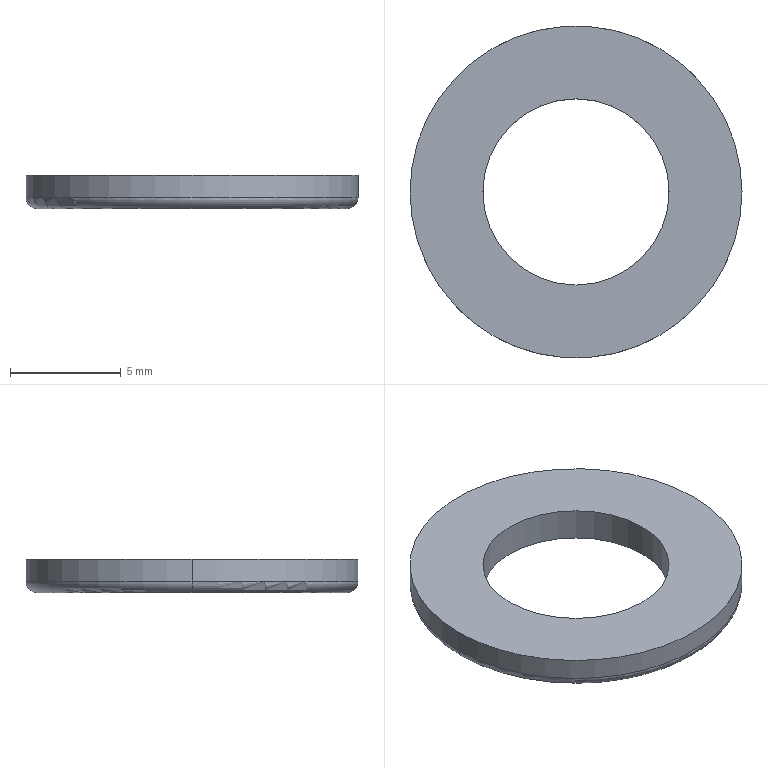Part | NX | features BREP 1 | 1 solid | 8 faces | box 15 x 15 x 1.5 mm | volume 179.214 mm3 | cylinder 4 | torus 2 | plane 2 | commonest cylinder face diameters 8.412 x2 15 x2
STEP:
#1=CARTESIAN_POINT('',(7.5,0.,6.));
#2=VERTEX_POINT('',#1);
#3=CARTESIAN_POINT('',(-7.5,0.,6.));
#4=VERTEX_POINT('',#3);
#5=CARTESIAN_POINT('',(0.,0.,6.));
#6=DIRECTION('',(0.,0.,-1.));
#7=DIRECTION('',(1.,0.,0.));
#8=AXIS2_PLACEMENT_3D('',#5,#6,#7);
#9=CIRCLE('',#8,7.5);
#10=EDGE_CURVE('',#2,#4,#9,.T.);
#11=ORIENTED_EDGE('',*,*,#10,.F.);
#12=CARTESIAN_POINT('',(7.5,0.,7.));
#13=VERTEX_POINT('',#12);
#14=CARTESIAN_POINT('',(7.5,0.,7.));
#15=DIRECTION('',(0.,0.,-1.));
#16=VECTOR('',#15,1000.);
#17=LINE('',#14,#16);
#18=EDGE_CURVE('',#13,#2,#17,.T.);
#19=ORIENTED_EDGE('',*,*,#18,.F.);
#20=CARTESIAN_POINT('',(-7.5,0.,7.));
#21=VERTEX_POINT('',#20);
#22=CARTESIAN_POINT('',(0.,0.,7.));
#23=DIRECTION('',(0.,0.,1.));
#24=DIRECTION('',(-1.,0.,0.));
#25=AXIS2_PLACEMENT_3D('',#22,#23,#24);
#26=CIRCLE('',#25,7.5);
#27=EDGE_CURVE('',#21,#13,#26,.T.);
#28=ORIENTED_EDGE('',*,*,#27,.F.);
#29=CARTESIAN_POINT('',(-7.5,0.,7.));
#30=DIRECTION('',(0.,0.,-1.));
#31=VECTOR('',#30,1000.);
#32=LINE('',#29,#31);
#33=EDGE_CURVE('',#21,#4,#32,.T.);
#34=ORIENTED_EDGE('',*,*,#33,.T.);
#35=EDGE_LOOP('',(#11,#19,#28,#34));
#36=FACE_BOUND('',#35,.T.);
#37=CARTESIAN_POINT('',(0.,0.,5.5));
#38=DIRECTION('',(0.,0.,1.));
#39=DIRECTION('',(-1.,0.,0.));
#40=AXIS2_PLACEMENT_3D('',#37,#38,#39);
#41=CYLINDRICAL_SURFACE('',#40,7.5);
#42=ADVANCED_FACE('',(#36),#41,.T.);
#43=ORIENTED_EDGE('',*,*,#33,.F.);
#44=CARTESIAN_POINT('',(0.,0.,7.));
#45=DIRECTION('',(0.,0.,1.));
#46=DIRECTION('',(1.,0.,0.));
#47=AXIS2_PLACEMENT_3D('',#44,#45,#46);
#48=CIRCLE('',#47,7.5);
#49=EDGE_CURVE('',#13,#21,#48,.T.);
#50=ORIENTED_EDGE('',*,*,#49,.F.);
#51=ORIENTED_EDGE('',*,*,#18,.T.);
#52=CARTESIAN_POINT('',(0.,0.,6.));
#53=DIRECTION('',(0.,0.,-1.));
#54=DIRECTION('',(-1.,0.,0.));
#55=AXIS2_PLACEMENT_3D('',#52,#53,#54);
#56=CIRCLE('',#55,7.5);
#57=EDGE_CURVE('',#4,#2,#56,.T.);
#58=ORIENTED_EDGE('',*,*,#57,.F.);
#59=EDGE_LOOP('',(#43,#50,#51,#58));
#60=FACE_BOUND('',#59,.T.);
#61=CARTESIAN_POINT('',(0.,0.,5.5));
#62=DIRECTION('',(0.,0.,1.));
#63=DIRECTION('',(-1.,0.,0.));
#64=AXIS2_PLACEMENT_3D('',#61,#62,#63);
#65=CYLINDRICAL_SURFACE('',#64,7.5);
#66=ADVANCED_FACE('',(#60),#65,.T.);
#67=CARTESIAN_POINT('',(7.,0.,5.5));
#68=VERTEX_POINT('',#67);
#69=CARTESIAN_POINT('',(7.,0.,6.));
#70=DIRECTION('',(0.,-1.,0.));
#71=DIRECTION('',(0.,0.,-1.));
#72=AXIS2_PLACEMENT_3D('',#69,#70,#71);
#73=CIRCLE('',#72,0.5);
#74=EDGE_CURVE('',#68,#2,#73,.T.);
#75=ORIENTED_EDGE('',*,*,#74,.F.);
#76=CARTESIAN_POINT('',(-7.,0.,5.5));
#77=VERTEX_POINT('',#76);
#78=CARTESIAN_POINT('',(0.,0.,5.5));
#79=DIRECTION('',(0.,0.,-1.));
#80=DIRECTION('',(-1.,0.,0.));
#81=AXIS2_PLACEMENT_3D('',#78,#79,#80);
#82=CIRCLE('',#81,7.);
#83=EDGE_CURVE('',#77,#68,#82,.T.);
#84=ORIENTED_EDGE('',*,*,#83,.F.);
#85=CARTESIAN_POINT('',(-7.,0.,6.));
#86=DIRECTION('',(0.,1.,0.));
#87=DIRECTION('',(0.,0.,-1.));
#88=AXIS2_PLACEMENT_3D('',#85,#86,#87);
#89=CIRCLE('',#88,0.5);
#90=EDGE_CURVE('',#77,#4,#89,.T.);
#91=ORIENTED_EDGE('',*,*,#90,.T.);
#92=ORIENTED_EDGE('',*,*,#57,.T.);
#93=EDGE_LOOP('',(#75,#84,#91,#92));
#94=FACE_BOUND('',#93,.T.);
#95=CARTESIAN_POINT('',(0.,0.,6.));
#96=DIRECTION('',(0.,0.,-1.));
#97=DIRECTION('',(1.,0.,0.));
#98=AXIS2_PLACEMENT_3D('',#95,#96,#97);
#99=TOROIDAL_SURFACE('',#98,7.,0.5);
#100=ADVANCED_FACE('',(#94),#99,.T.);
#101=ORIENTED_EDGE('',*,*,#10,.T.);
#102=ORIENTED_EDGE('',*,*,#90,.F.);
#103=CARTESIAN_POINT('',(0.,0.,5.5));
#104=DIRECTION('',(0.,0.,-1.));
#105=DIRECTION('',(1.,0.,0.));
#106=AXIS2_PLACEMENT_3D('',#103,#104,#105);
#107=CIRCLE('',#106,7.);
#108=EDGE_CURVE('',#68,#77,#107,.T.);
#109=ORIENTED_EDGE('',*,*,#108,.F.);
#110=ORIENTED_EDGE('',*,*,#74,.T.);
#111=EDGE_LOOP('',(#101,#102,#109,#110));
#112=FACE_BOUND('',#111,.T.);
#113=CARTESIAN_POINT('',(0.,0.,6.));
#114=DIRECTION('',(0.,0.,-1.));
#115=DIRECTION('',(1.,0.,0.));
#116=AXIS2_PLACEMENT_3D('',#113,#114,#115);
#117=TOROIDAL_SURFACE('',#116,7.,0.5);
#118=ADVANCED_FACE('',(#112),#117,.T.);
#119=ORIENTED_EDGE('',*,*,#108,.T.);
#120=ORIENTED_EDGE('',*,*,#83,.T.);
#121=EDGE_LOOP('',(#119,#120));
#122=FACE_BOUND('',#121,.T.);
#123=CARTESIAN_POINT('',(4.206,0.,5.5));
#124=VERTEX_POINT('',#123);
#125=CARTESIAN_POINT('',(-4.206,0.,5.5));
#126=VERTEX_POINT('',#125);
#127=CARTESIAN_POINT('',(0.,0.,5.5));
#128=DIRECTION('',(0.,0.,1.));
#129=DIRECTION('',(1.,0.,0.));
#130=AXIS2_PLACEMENT_3D('',#127,#128,#129);
#131=CIRCLE('',#130,4.206);
#132=EDGE_CURVE('',#124,#126,#131,.T.);
#133=ORIENTED_EDGE('',*,*,#132,.T.);
#134=CARTESIAN_POINT('',(0.,0.,5.5));
#135=DIRECTION('',(0.,0.,1.));
#136=DIRECTION('',(-1.,0.,0.));
#137=AXIS2_PLACEMENT_3D('',#134,#135,#136);
#138=CIRCLE('',#137,4.206);
#139=EDGE_CURVE('',#126,#124,#138,.T.);
#140=ORIENTED_EDGE('',*,*,#139,.T.);
#141=EDGE_LOOP('',(#133,#140));
#142=FACE_BOUND('',#141,.T.);
#143=CARTESIAN_POINT('',(0.,0.,5.5));
#144=DIRECTION('',(0.,0.,-1.));
#145=DIRECTION('',(1.,0.,0.));
#146=AXIS2_PLACEMENT_3D('',#143,#144,#145);
#147=PLANE('',#146);
#148=ADVANCED_FACE('',(#122,#142),#147,.T.);
#149=CARTESIAN_POINT('',(-4.206,0.,7.));
#150=VERTEX_POINT('',#149);
#151=CARTESIAN_POINT('',(-4.206,0.,7.));
#152=DIRECTION('',(0.,0.,-1.));
#153=VECTOR('',#152,1000.);
#154=LINE('',#151,#153);
#155=EDGE_CURVE('',#126,#150,#154,.F.);
#156=ORIENTED_EDGE('',*,*,#155,.T.);
#157=CARTESIAN_POINT('',(4.206,0.,7.));
#158=VERTEX_POINT('',#157);
#159=CARTESIAN_POINT('',(0.,0.,7.));
#160=DIRECTION('',(0.,0.,-1.));
#161=DIRECTION('',(1.,0.,0.));
#162=AXIS2_PLACEMENT_3D('',#159,#160,#161);
#163=CIRCLE('',#162,4.206);
#164=EDGE_CURVE('',#158,#150,#163,.T.);
#165=ORIENTED_EDGE('',*,*,#164,.F.);
#166=CARTESIAN_POINT('',(4.206,0.,7.));
#167=DIRECTION('',(0.,0.,-1.));
#168=VECTOR('',#167,1000.);
#169=LINE('',#166,#168);
#170=EDGE_CURVE('',#124,#158,#169,.F.);
#171=ORIENTED_EDGE('',*,*,#170,.F.);
#172=ORIENTED_EDGE('',*,*,#139,.F.);
#173=EDGE_LOOP('',(#156,#165,#171,#172));
#174=FACE_BOUND('',#173,.T.);
#175=CARTESIAN_POINT('',(0.,0.,5.5));
#176=DIRECTION('',(0.,0.,1.));
#177=DIRECTION('',(-1.,0.,0.));
#178=AXIS2_PLACEMENT_3D('',#175,#176,#177);
#179=CYLINDRICAL_SURFACE('',#178,4.206);
#180=ADVANCED_FACE('',(#174),#179,.F.);
#181=ORIENTED_EDGE('',*,*,#132,.F.);
#182=ORIENTED_EDGE('',*,*,#170,.T.);
#183=CARTESIAN_POINT('',(0.,0.,7.));
#184=DIRECTION('',(0.,0.,-1.));
#185=DIRECTION('',(-1.,0.,0.));
#186=AXIS2_PLACEMENT_3D('',#183,#184,#185);
#187=CIRCLE('',#186,4.206);
#188=EDGE_CURVE('',#150,#158,#187,.T.);
#189=ORIENTED_EDGE('',*,*,#188,.F.);
#190=ORIENTED_EDGE('',*,*,#155,.F.);
#191=EDGE_LOOP('',(#181,#182,#189,#190));
#192=FACE_BOUND('',#191,.T.);
#193=CARTESIAN_POINT('',(0.,0.,5.5));
#194=DIRECTION('',(0.,0.,1.));
#195=DIRECTION('',(-1.,0.,0.));
#196=AXIS2_PLACEMENT_3D('',#193,#194,#195);
#197=CYLINDRICAL_SURFACE('',#196,4.206);
#198=ADVANCED_FACE('',(#192),#197,.F.);
#199=ORIENTED_EDGE('',*,*,#49,.T.);
#200=ORIENTED_EDGE('',*,*,#27,.T.);
#201=EDGE_LOOP('',(#199,#200));
#202=FACE_BOUND('',#201,.T.);
#203=ORIENTED_EDGE('',*,*,#188,.T.);
#204=ORIENTED_EDGE('',*,*,#164,.T.);
#205=EDGE_LOOP('',(#203,#204));
#206=FACE_BOUND('',#205,.T.);
#207=CARTESIAN_POINT('',(0.,0.,7.));
#208=DIRECTION('',(0.,0.,-1.));
#209=DIRECTION('',(1.,0.,0.));
#210=AXIS2_PLACEMENT_3D('',#207,#208,#209);
#211=PLANE('',#210);
#212=ADVANCED_FACE('',(#202,#206),#211,.F.);
#213=CLOSED_SHELL('',(#42,#66,#100,#118,#148,#180,#198,#212));
#214=MANIFOLD_SOLID_BREP('',#213);
#215=(LENGTH_UNIT()NAMED_UNIT(*)SI_UNIT(.MILLI.,.METRE.));
#216=UNCERTAINTY_MEASURE_WITH_UNIT(LENGTH_MEASURE(0.00001),#215,'','');
#217=(NAMED_UNIT(*)PLANE_ANGLE_UNIT()SI_UNIT($,.RADIAN.));
#218=(NAMED_UNIT(*)SI_UNIT($,.STERADIAN.)SOLID_ANGLE_UNIT());
#219=(GEOMETRIC_REPRESENTATION_CONTEXT(3)GLOBAL_UNCERTAINTY_ASSIGNED_CONTEXT((#216))GLOBAL_UNIT_ASSIGNED_CONTEXT((#215,#217,#218))REPRESENTATION_CONTEXT('',''));
#220=ADVANCED_BREP_SHAPE_REPRESENTATION('',(#214),#219);